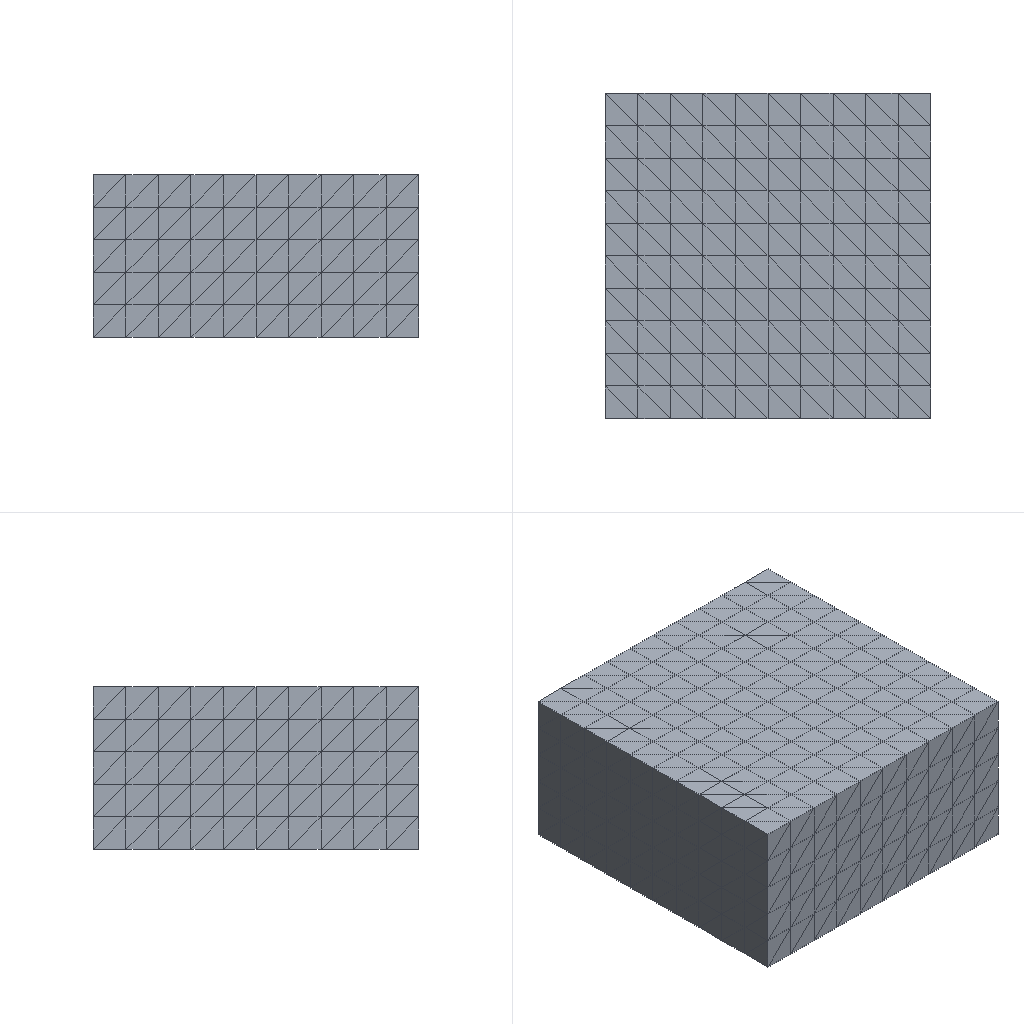Simulation study | abaqus
Notes in the study folder:
17 contact-proxy block compression
job_status=None
Umax_mm=0.000329537
S_Mises_max_MPa=5.03414
Set-up summary:
category,name,step,type,value,unit,region
solver,abaqus,,Abaqus/CAE 2024
units,mm-N-s-tonne (MPa),,inferred,E=210000 density=7.85e-09
analysis,Step-1,,static,time_period=1
mesh,nodes,,,5678
mesh,elements,,,3627
element_type,C3D10,,,3627
material,Steel,,E,210000
material,Steel,,nu,0.3
material,Steel,,density,7.85e-09
section,Steel,,solid section,,,_PickedSet2
load,Load,Step-1,pressure,3,,TOP
bc,BC,Step-1,encastre,[dofs=ENCASTRE],,FIXED
Abaqus input file, long lists of numbers shortened:
*Heading
** Job name: deck Model name: M17
** Generated by: Abaqus/CAE 2024
*Preprint, echo=NO, model=NO, history=NO, contact=NO
**
** PARTS
**
*Part, name=P
*Node
      1,          20.,          20.,          20.
      2,          20.,         -20.,          20.
** (5676 more lines like these left out)
*Element, type=C3D10
   1,  403,  404,  405,  406,  829,  828,  827,  831,  830,  832
   2,  404,  407,  405,  408,  834,  833,  828,  836,  835,  837
** (3625 more lines like these left out)
*Nset, nset=_PickedSet2, internal, generate
    1,  5678,     1
*Elset, elset=_PickedSet2, internal, generate
    1,  3627,     1
** Section: Sec
*Solid Section, elset=_PickedSet2, material=Steel
,
*End Part
**
**
** ASSEMBLY
**
*Assembly, name=Assembly
**
*Instance, name=I, part=P
*End Instance
**
*Nset, nset=FIXED, instance=I
    3,    4,    6,    7,   22,   23,   24,   25,   26,   27,   28,   29,   30,   48,   49,   50
   51,   52,   53,   54,   55,   56,   57,   58,   59,   60,   61,   62,   63,   64,   65,   66
** (26 more lines like these left out)
*Elset, elset=FIXED, instance=I
   57,  143,  192,  454,  582,  746,  914,  936, 1047, 1111, 1156, 1175, 1312, 1397, 1631, 1635
 1637, 1642, 1750, 1810, 1817, 1854, 1865, 1887, 1909, 1933, 1967, 1970, 1980, 1982, 1984, 1987
** (11 more lines like these left out)
*Elset, elset=_TOP_S3, internal, instance=I
  102,  118,  167,  179,  206,  210,  276,  321,  332,  379,  410,  519,  557,  583,  600,  630
  672,  691,  737,  767,  803,  804,  814,  867,  900,  938,  956,  959,  982, 1003, 1118, 1276
** (10 more lines like these left out)
*Elset, elset=_TOP_S4, internal, instance=I
  140, 2859, 2913, 3142, 3241, 3357
*Elset, elset=_TOP_S1, internal, instance=I
  217,  666, 2681
*Elset, elset=_TOP_S2, internal, instance=I
 1802, 2602, 2625
*Surface, type=ELEMENT, name=TOP
_TOP_S3, S3
_TOP_S4, S4
_TOP_S2, S2
_TOP_S1, S1
*End Assembly
**
** MATERIALS
**
*Material, name=Steel
*Density
 7.85e-09,
*Elastic
210000., 0.3
** ----------------------------------------------------------------
**
** STEP: Step-1
**
*Step, name=Step-1, nlgeom=NO
*Static
1., 1., 1e-05, 1.
**
** BOUNDARY CONDITIONS
**
** Name: BC Type: Symmetry/Antisymmetry/Encastre
*Boundary
FIXED, ENCASTRE
**
** LOADS
**
** Name: Load   Type: Pressure
*Dsload
TOP, P, 3.
**
** OUTPUT REQUESTS
**
*Restart, write, frequency=0
**
** FIELD OUTPUT: F-Output-1
**
*Output, field, variable=PRESELECT
**
** HISTORY OUTPUT: H-Output-1
**
*Output, history, variable=PRESELECT
*End Step
Results summary:
result,odb.job_status,,,JOB_STATUS_COMPLETED_SUCCESSFULLY,"consistent, unstated (Abaqus has no unit system)"
result,steps[0].procedure,Step-1,,*STATIC,"consistent, unstated (Abaqus has no unit system)"
result,steps[0].time_period,Step-1,,1,"consistent, unstated (Abaqus has no unit system)"
result,steps[0].n_frames,Step-1,,2,"consistent, unstated (Abaqus has no unit system)"
result,steps[0].last_frame.id,Step-1,,1,"consistent, unstated (Abaqus has no unit system)"
result,steps[0].last_frame.value,Step-1,,1,"consistent, unstated (Abaqus has no unit system)"
result,steps[0].last_frame.description,Step-1,,Increment      1: Step Time =    1.000,"consistent, unstated (Abaqus has no unit system)"
result,steps[0].completed,Step-1,,True,"consistent, unstated (Abaqus has no unit system)"
result,steps[0].max_U_magnitude,Step-1,,0.0003295,"consistent, unstated (Abaqus has no unit system)"
result,steps[0].max_S_mises,Step-1,,5.034,"consistent, unstated (Abaqus has no unit system)"
result,steps[0].RF_sum[1],Step-1,,2.42293e-05,"consistent, unstated (Abaqus has no unit system)"
result,steps[0].RF_sum[2],Step-1,,5.36442e-07,"consistent, unstated (Abaqus has no unit system)"
result,steps[0].RF_sum[3],Step-1,,4800,"consistent, unstated (Abaqus has no unit system)"
result,steps[1].procedure,Step-1,,*STATIC,"consistent, unstated (Abaqus has no unit system)"
result,steps[1].time_period,Step-1,,1,"consistent, unstated (Abaqus has no unit system)"
result,steps[1].n_frames,Step-1,,2,"consistent, unstated (Abaqus has no unit system)"
result,steps[1].last_frame.id,Step-1,,1,"consistent, unstated (Abaqus has no unit system)"
result,steps[1].last_frame.value,Step-1,,1,"consistent, unstated (Abaqus has no unit system)"
result,steps[1].last_frame.description,Step-1,,Increment      1: Step Time =    1.000,"consistent, unstated (Abaqus has no unit system)"
result,steps[1].completed,Step-1,,True,"consistent, unstated (Abaqus has no unit system)"
result,steps[1].max_U_magnitude,Step-1,,0.0003295,"consistent, unstated (Abaqus has no unit system)"
result,steps[1].max_S_mises,Step-1,,5.034,"consistent, unstated (Abaqus has no unit system)"
result,steps[1].RF_sum[1],Step-1,,2.42293e-05,"consistent, unstated (Abaqus has no unit system)"
result,steps[1].RF_sum[2],Step-1,,5.36442e-07,"consistent, unstated (Abaqus has no unit system)"
result,steps[1].RF_sum[3],Step-1,,4800,"consistent, unstated (Abaqus has no unit system)"